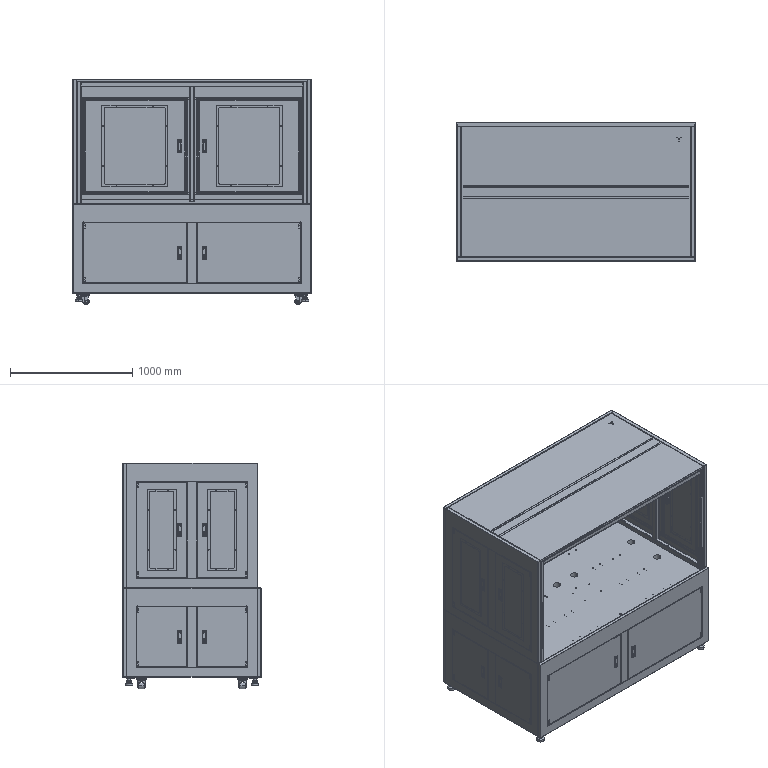Part | SolidWorks | features ReferencePattern 27, LocalLPattern 6, MirrorCompFeat 6 | 183 solids | 9647 faces | volume 240689348 mm3 | plane 5179 | cylinder 3412 | spline 672 | cone 384 | commonest cylinder face diameters 4 x879 1 x409 8 x236 2 x210 3 x166 5 x112